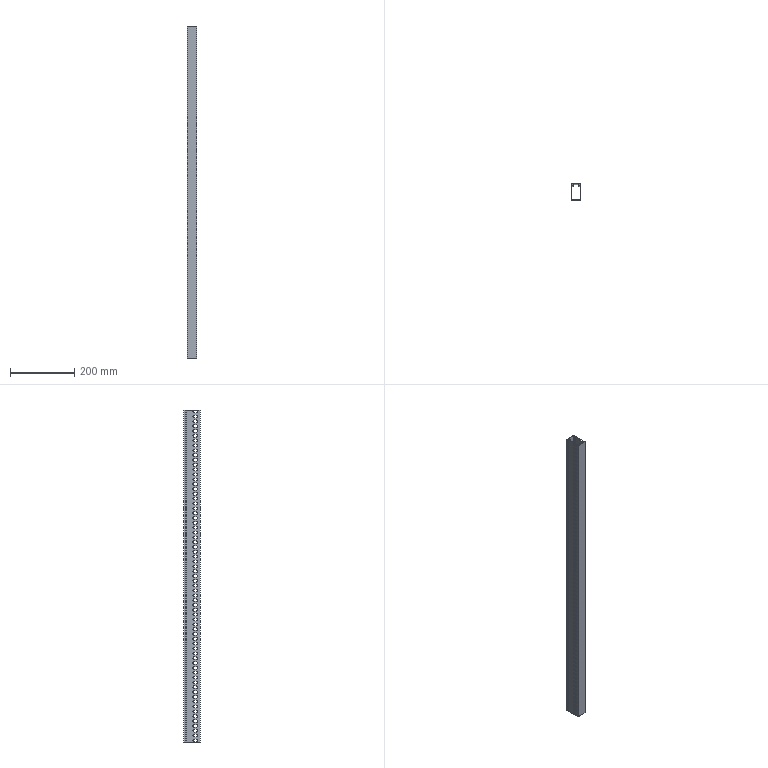Part | SolidWorks | features BaseBody 1 | 1 solid | 578 faces | box 30 x 50 x 1030 mm | volume 167719 mm3 | plane 302 | cylinder 276 | commonest cylinder face diameters 8 x276